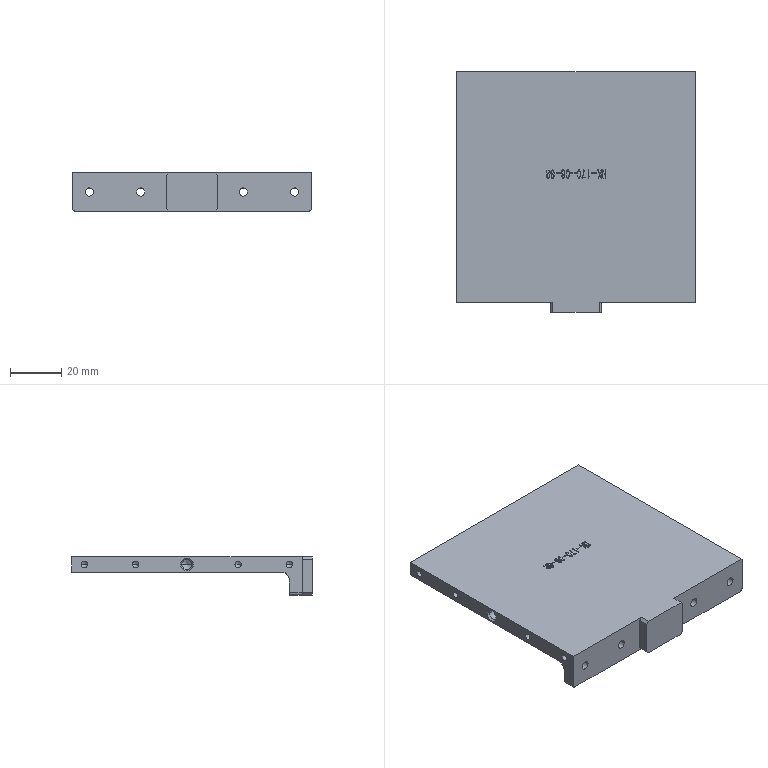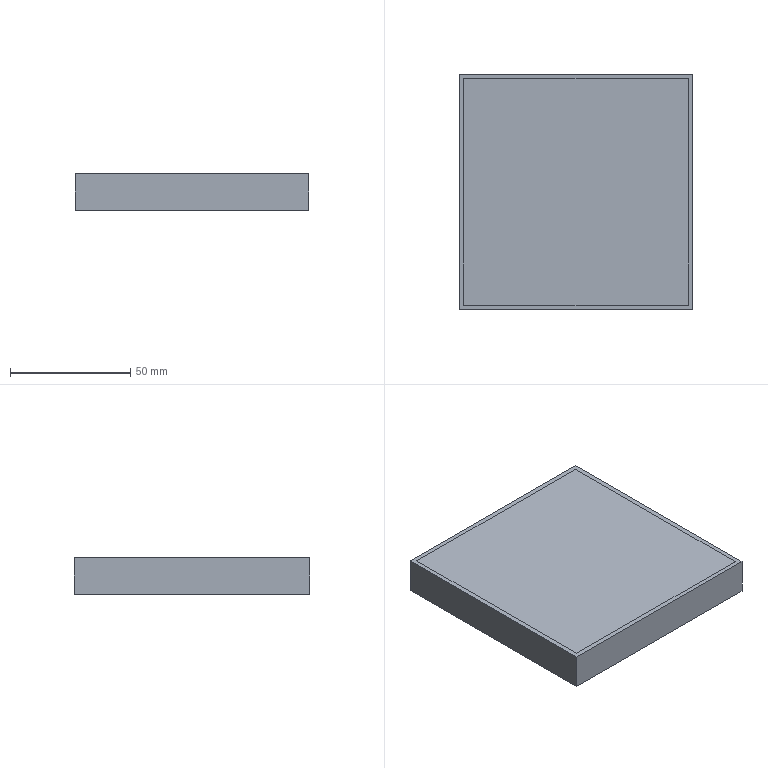CAM job | NX | 3+2 milling, drilling | part box 93.2 x 94 x 15 mm | stock box 97.2 x 98 x 15 mm
Tools:
number,name,description,diameter,corner_radius,flute_length,length,flutes
15,D10,Milling Tool-5 Parameters,10.0,0.0,50.0,75.0,2
1,D6A45,Milling Tool-5 Parameters,6.0,0.0,50.0,75.0,2
14,D10JING,Milling Tool-5 Parameters,10.0,0.0,50.0,75.0,2
16,D4R0.5,Milling Tool-5 Parameters,4.0,0.5,50.0,75.0,2
3,3.3ZT,Drilling Tool,3.3,0.0,35.0,50.0,2
2,2.5ZT,Drilling Tool,2.5,0.0,35.0,50.0,2
17,D3,Milling Tool-5 Parameters,3.0,0.0,50.0,75.0,2
Operations:
program,operation,operation_type,tool,method,geometry_group,spindle_rpm,surface_speed,feed_per_tooth,feed_cut,feed_plunge,cut_length_mm,path_length_mm,cut_time_min,machine_time_min
1,ZLEVEL_PROFILE_COPY_1_COPY,ZLevelMilling,D10,METHOD,A,9500.0,298.0,0.1579,3000.0,1000.0,10098.442,10169.842,3.393,3.4
1,PLANAR_MILL_COPY_COPY_COPY_COPY_COPY,PlanarMilling,D6A45,METHOD,A,9500.0,179.0,0.0658,1250.0,100.0,384.377,443.377,0.3075,0.3134
1,ZLEVEL_PROFILE_COPY_1_COPY_COPY_1,ZLevelMilling,D10JING,METHOD,A,9500.0,298.0,0.0632,1200.0,1000.0,2015.846,2103.271,1.681,1.689
2,FLOOR_WALL,VolumeBased25DMillingOperation,D10,METHOD,B,9500.0,298.0,0.1579,3000.0,1000.0,8659.368,8731.168,2.89,2.898
2,FLOOR_WALL_1,VolumeBased25DMillingOperation,D10,METHOD,B,9500.0,298.0,0.1579,3000.0,1000.0,2534.386,2677.914,0.9797,0.9941
2,FLOOR_WALL_COPY,VolumeBased25DMillingOperation,D10JING,METHOD,B,9500.0,298.0,0.0789,1500.0,1000.0,2984.225,3300.484,1.992,2.024
2,ZLEVEL_PROFILE,ZLevelMilling,D4R0.5,METHOD,B,9500.0,119.0,0.1579,3000.0,1000.0,10553.69,10619.79,3.52,3.526
2,ZLEVEL_PROFILE_COPY,ZLevelMilling,D4R0.5,METHOD,B,9500.0,119.0,0.1579,3000.0,1000.0,483.656,697.919,0.1646,0.186
2,PLANAR_MILL_COPY_COPY_COPY_COPY_COPY_COPY,PlanarMilling,D6A45,METHOD,B,9500.0,179.0,0.0658,1250.0,100.0,512.011,750.115,0.4096,0.4334
2,PLANAR_MILL_COPY_COPY_COPY_COPY_COPY_COPY_1,PlanarMilling,D6A45,METHOD,B,9500.0,179.0,0.0658,1250.0,100.0,214.377,273.377,0.1715,0.1774
3,DRILLING_COPY,Operation,D6A45,METHOD,C,5000.0,94.0,0.035,350.0,0.0,19.0,195.56,0.0543,0.0719
3,DRILLING_COPY_1_COPY,Operation,3.3ZT,METHOD,C,2000.0,21.0,0.05,200.0,0.0,46.361,250.281,0.2318,0.2522
3,PLANAR_MILL_COPY_COPY_COPY_COPY_COPY_COPY_1_COPY,PlanarMilling,D6A45,METHOD,C,9500.0,179.0,0.0658,1250.0,100.0,78.406,137.406,0.0627,0.0686
3,刀补,ZLevelMilling,D10JING,METHOD,C,9500.0,298.0,0.0632,1200.0,1000.0,257.031,952.936,0.2191,0.2886
4,DRILLING_COPY_COPY,Operation,D6A45,METHOD,D,5000.0,94.0,0.035,350.0,0.0,23.0,198.895,0.0657,0.0833
4,DRILLING_COPY_1_COPY_COPY,Operation,2.5ZT,METHOD,D,2000.0,21.0,0.05,200.0,0.0,49.004,247.568,0.245,0.2649
4,HOLE_MILLING,CylinderMilling,D3,METHOD,D,9500.0,89.0,0.0526,1000.0,100.0,117.225,185.225,0.1172,0.124
4,DRILLING_COPY_COPY_COPY,Operation,D6A45,METHOD,D,5000.0,94.0,0.035,350.0,0.0,5.5,71.0,0.0157,0.0223
4,HOLE_MILLING_COPY,CylinderMilling,D3,METHOD,D,9500.0,89.0,0.0526,1000.0,100.0,19.811,87.811,0.0198,0.0266